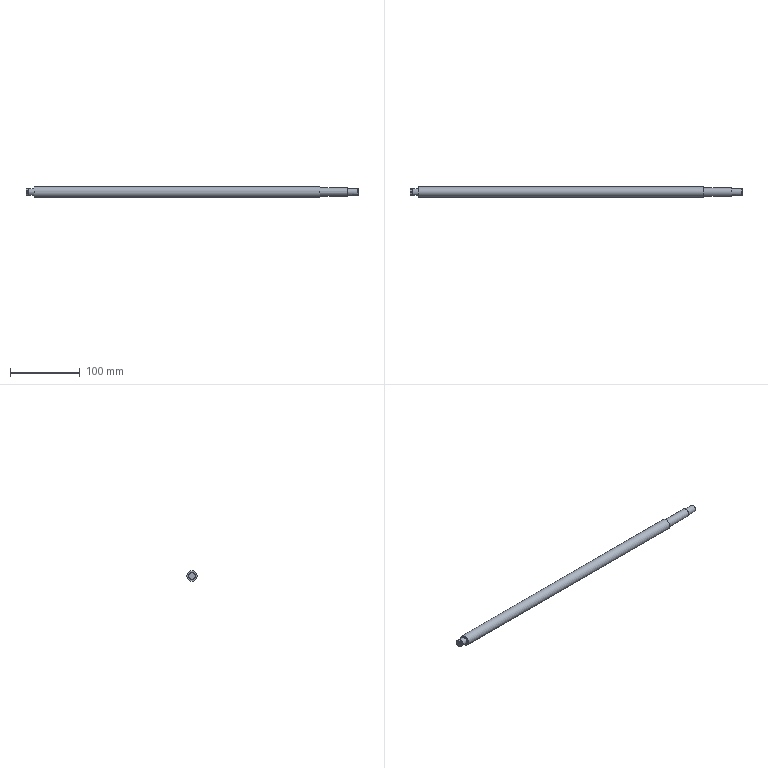Part | STEP file | 1 solid | 17 faces | box 475 x 15 x 15 mm | volume 78728 mm3 | plane 7 | cylinder 6 | spline 2 | cone 2 | commonest cylinder face diameters 10 x3 9.6 x1 12 x1 15 x1
STEP:
#1=CARTESIAN_POINT('',(0.,0.,0.));
#2=DIRECTION('',(0.,0.,1.));
#3=DIRECTION('',(1.,0.,0.));
#4=AXIS2_PLACEMENT_3D('',#1,#2,#3);
#5=CARTESIAN_POINT('',(12.,0.,7.5));
#6=VERTEX_POINT('',#5);
#7=CARTESIAN_POINT('',(12.,0.,0.));
#8=DIRECTION('',(1.,0.,0.));
#9=DIRECTION('',(0.,0.,1.));
#10=AXIS2_PLACEMENT_3D('',#7,#8,#9);
#11=CIRCLE('',#10,7.5);
#12=CARTESIAN_POINT('',(0.,0.,0.));
#13=DIRECTION('',(-1.,0.,0.));
#14=DIRECTION('',(0.,0.,1.));
#15=AXIS2_PLACEMENT_3D('',#12,#13,#14);
#16=CYLINDRICAL_SURFACE('',#15,7.5);
#17=CARTESIAN_POINT('',(6.283,-12.));
#18=DIRECTION('',(-1.,0.));
#19=VECTOR('',#18,1.);
#20=LINE('',#17,#19);
#21=(GEOMETRIC_REPRESENTATION_CONTEXT(2)PARAMETRIC_REPRESENTATION_CONTEXT()REPRESENTATION_CONTEXT('',''));
#22=DEFINITIONAL_REPRESENTATION('',(#20),#21);
#23=PCURVE('',#16,#22);
#24=CARTESIAN_POINT('',(12.,5.,0.));
#25=DIRECTION('',(1.,0.,0.));
#26=DIRECTION('',(0.,0.,-1.));
#27=AXIS2_PLACEMENT_3D('',#24,#25,#26);
#28=PLANE('',#27);
#29=CARTESIAN_POINT('',(0.,-5.));
#30=DIRECTION('',(-1.,0.));
#31=AXIS2_PLACEMENT_2D('',#29,#30);
#32=CIRCLE('',#31,7.5);
#33=(GEOMETRIC_REPRESENTATION_CONTEXT(2)PARAMETRIC_REPRESENTATION_CONTEXT()REPRESENTATION_CONTEXT('',''));
#34=DEFINITIONAL_REPRESENTATION('',(#32),#33);
#35=PCURVE('',#28,#34);
#36=SURFACE_CURVE('',#11,(#23,#35),.PCURVE_S1.);
#37=EDGE_CURVE('',#6,#6,#36,.T.);
#38=ORIENTED_EDGE('',*,*,#37,.T.);
#39=CARTESIAN_POINT('',(420.,0.,7.5));
#40=VERTEX_POINT('',#39);
#41=CARTESIAN_POINT('',(420.,0.,7.5));
#42=CARTESIAN_POINT('',(12.,0.,7.5));
#43=B_SPLINE_CURVE_WITH_KNOTS('',1,(#41,#42),.UNSPECIFIED.,.F.,.F.,(2,2),(-420.,-12.),.PIECEWISE_BEZIER_KNOTS.);
#44=CARTESIAN_POINT('',(0.,0.));
#45=DIRECTION('',(0.,1.));
#46=VECTOR('',#45,1.);
#47=LINE('',#44,#46);
#48=(GEOMETRIC_REPRESENTATION_CONTEXT(2)PARAMETRIC_REPRESENTATION_CONTEXT()REPRESENTATION_CONTEXT('',''));
#49=DEFINITIONAL_REPRESENTATION('',(#47),#48);
#50=PCURVE('',#16,#49);
#51=CARTESIAN_POINT('',(6.283,0.));
#52=DIRECTION('',(0.,1.));
#53=VECTOR('',#52,1.);
#54=LINE('',#51,#53);
#55=(GEOMETRIC_REPRESENTATION_CONTEXT(2)PARAMETRIC_REPRESENTATION_CONTEXT()REPRESENTATION_CONTEXT('',''));
#56=DEFINITIONAL_REPRESENTATION('',(#54),#55);
#57=PCURVE('',#16,#56);
#58=SEAM_CURVE('',#43,(#50,#57),.PCURVE_S1.);
#59=EDGE_CURVE('',#40,#6,#58,.T.);
#60=ORIENTED_EDGE('',*,*,#59,.F.);
#61=CARTESIAN_POINT('',(420.,0.,0.));
#62=DIRECTION('',(-1.,0.,0.));
#63=DIRECTION('',(0.,0.,1.));
#64=AXIS2_PLACEMENT_3D('',#61,#62,#63);
#65=CIRCLE('',#64,7.5);
#66=CARTESIAN_POINT('',(0.,-420.));
#67=DIRECTION('',(1.,0.));
#68=VECTOR('',#67,1.);
#69=LINE('',#66,#68);
#70=(GEOMETRIC_REPRESENTATION_CONTEXT(2)PARAMETRIC_REPRESENTATION_CONTEXT()REPRESENTATION_CONTEXT('',''));
#71=DEFINITIONAL_REPRESENTATION('',(#69),#70);
#72=PCURVE('',#16,#71);
#73=CARTESIAN_POINT('',(420.,6.,0.));
#74=DIRECTION('',(-1.,0.,0.));
#75=DIRECTION('',(0.,0.,1.));
#76=AXIS2_PLACEMENT_3D('',#73,#74,#75);
#77=PLANE('',#76);
#78=CARTESIAN_POINT('',(0.,-6.));
#79=DIRECTION('',(1.,0.));
#80=AXIS2_PLACEMENT_2D('',#78,#79);
#81=CIRCLE('',#80,7.5);
#82=(GEOMETRIC_REPRESENTATION_CONTEXT(2)PARAMETRIC_REPRESENTATION_CONTEXT()REPRESENTATION_CONTEXT('',''));
#83=DEFINITIONAL_REPRESENTATION('',(#81),#82);
#84=PCURVE('',#77,#83);
#85=SURFACE_CURVE('',#65,(#72,#84),.PCURVE_S1.);
#86=EDGE_CURVE('',#40,#40,#85,.T.);
#87=ORIENTED_EDGE('',*,*,#86,.T.);
#88=ORIENTED_EDGE('',*,*,#59,.T.);
#89=EDGE_LOOP('',(#38,#60,#87,#88));
#90=FACE_BOUND('',#89,.T.);
#91=ADVANCED_FACE('',(#90),#16,.T.);
#92=CARTESIAN_POINT('',(12.,0.,-5.3));
#93=VERTEX_POINT('',#92);
#94=CARTESIAN_POINT('',(12.,0.,5.3));
#95=VERTEX_POINT('',#94);
#96=CARTESIAN_POINT('',(12.,0.,-5.3));
#97=CARTESIAN_POINT('',(12.,-10.6,-5.3));
#98=CARTESIAN_POINT('',(12.,-10.6,5.3));
#99=CARTESIAN_POINT('',(12.,0.,5.3));
#100=(BOUNDED_CURVE()B_SPLINE_CURVE(3,(#96,#97,#98,#99),.UNSPECIFIED.,.F.,.F.)B_SPLINE_CURVE_WITH_KNOTS((4,4),(0.,1.),.PIECEWISE_BEZIER_KNOTS.)CURVE()GEOMETRIC_REPRESENTATION_ITEM()RATIONAL_B_SPLINE_CURVE((1.,0.3333,0.3333,1.))REPRESENTATION_ITEM(''));
#101=CARTESIAN_POINT('',(5.3,-5.));
#102=CARTESIAN_POINT('',(5.3,-15.6));
#103=CARTESIAN_POINT('',(-5.3,-15.6));
#104=CARTESIAN_POINT('',(-5.3,-5.));
#105=(BOUNDED_CURVE()B_SPLINE_CURVE(3,(#101,#102,#103,#104),.UNSPECIFIED.,.F.,.F.)B_SPLINE_CURVE_WITH_KNOTS((4,4),(0.,1.),.PIECEWISE_BEZIER_KNOTS.)CURVE()GEOMETRIC_REPRESENTATION_ITEM()RATIONAL_B_SPLINE_CURVE((1.,0.3333,0.3333,1.))REPRESENTATION_ITEM(''));
#106=(GEOMETRIC_REPRESENTATION_CONTEXT(2)PARAMETRIC_REPRESENTATION_CONTEXT()REPRESENTATION_CONTEXT('',''));
#107=DEFINITIONAL_REPRESENTATION('',(#105),#106);
#108=PCURVE('',#28,#107);
#109=CARTESIAN_POINT('',(11.7,0.,-5.));
#110=CARTESIAN_POINT('',(11.7,10.,-5.));
#111=CARTESIAN_POINT('',(11.7,10.,5.));
#112=CARTESIAN_POINT('',(11.7,0.,5.));
#113=CARTESIAN_POINT('',(11.7,-10.,5.));
#114=CARTESIAN_POINT('',(11.7,-10.,-5.));
#115=CARTESIAN_POINT('',(11.7,0.,-5.));
#116=CARTESIAN_POINT('',(11.876,0.,-5.));
#117=CARTESIAN_POINT('',(11.876,10.,-5.));
#118=CARTESIAN_POINT('',(11.876,10.,5.));
#119=CARTESIAN_POINT('',(11.876,0.,5.));
#120=CARTESIAN_POINT('',(11.876,-10.,5.));
#121=CARTESIAN_POINT('',(11.876,-10.,-5.));
#122=CARTESIAN_POINT('',(11.876,0.,-5.));
#123=CARTESIAN_POINT('',(12.,0.,-5.124));
#124=CARTESIAN_POINT('',(12.,10.249,-5.124));
#125=CARTESIAN_POINT('',(12.,10.249,5.124));
#126=CARTESIAN_POINT('',(12.,0.,5.124));
#127=CARTESIAN_POINT('',(12.,-10.249,5.124));
#128=CARTESIAN_POINT('',(12.,-10.249,-5.124));
#129=CARTESIAN_POINT('',(12.,0.,-5.124));
#130=CARTESIAN_POINT('',(12.,0.,-5.3));
#131=CARTESIAN_POINT('',(12.,10.6,-5.3));
#132=CARTESIAN_POINT('',(12.,10.6,5.3));
#133=CARTESIAN_POINT('',(12.,0.,5.3));
#134=CARTESIAN_POINT('',(12.,-10.6,5.3));
#135=CARTESIAN_POINT('',(12.,-10.6,-5.3));
#136=CARTESIAN_POINT('',(12.,0.,-5.3));
#137=(BOUNDED_SURFACE()B_SPLINE_SURFACE(3,3,((#109,#110,#111,#112,#113,#114,#115),(#116,#117,#118,#119,#120,#121,#122),(#123,#124,#125,#126,#127,#128,#129),(#130,#131,#132,#133,#134,#135,#136)),.UNSPECIFIED.,.F.,.T.,.F.)B_SPLINE_SURFACE_WITH_KNOTS((4,4),(1,3,3,3,1),(0.,1.),(-0.5,0.,0.5,1.,1.5),.UNSPECIFIED.)GEOMETRIC_REPRESENTATION_ITEM()RATIONAL_B_SPLINE_SURFACE(((1.,0.3333,0.3333,1.,0.3333,0.3333,1.),(0.8047,0.2682,0.2682,0.8047,0.2682,0.2682,0.8047),(0.8047,0.2682,0.2682,0.8047,0.2682,0.2682,0.8047),(1.,0.3333,0.3333,1.,0.3333,0.3333,1.)))REPRESENTATION_ITEM('')SURFACE());
#138=CARTESIAN_POINT('',(1.,1.));
#139=CARTESIAN_POINT('',(1.,0.5));
#140=B_SPLINE_CURVE_WITH_KNOTS('',1,(#138,#139),.UNSPECIFIED.,.F.,.F.,(2,2),(0.,1.),.PIECEWISE_BEZIER_KNOTS.);
#141=(GEOMETRIC_REPRESENTATION_CONTEXT(2)PARAMETRIC_REPRESENTATION_CONTEXT()REPRESENTATION_CONTEXT('',''));
#142=DEFINITIONAL_REPRESENTATION('',(#140),#141);
#143=PCURVE('',#137,#142);
#144=SURFACE_CURVE('',#100,(#108,#143),.PCURVE_S1.);
#145=EDGE_CURVE('',#93,#95,#144,.T.);
#146=ORIENTED_EDGE('',*,*,#145,.F.);
#147=CARTESIAN_POINT('',(12.,0.,5.3));
#148=CARTESIAN_POINT('',(12.,10.6,5.3));
#149=CARTESIAN_POINT('',(12.,10.6,-5.3));
#150=CARTESIAN_POINT('',(12.,0.,-5.3));
#151=(BOUNDED_CURVE()B_SPLINE_CURVE(3,(#147,#148,#149,#150),.UNSPECIFIED.,.F.,.F.)B_SPLINE_CURVE_WITH_KNOTS((4,4),(0.,1.),.PIECEWISE_BEZIER_KNOTS.)CURVE()GEOMETRIC_REPRESENTATION_ITEM()RATIONAL_B_SPLINE_CURVE((1.,0.3333,0.3333,1.))REPRESENTATION_ITEM(''));
#152=CARTESIAN_POINT('',(-5.3,-5.));
#153=CARTESIAN_POINT('',(-5.3,5.6));
#154=CARTESIAN_POINT('',(5.3,5.6));
#155=CARTESIAN_POINT('',(5.3,-5.));
#156=(BOUNDED_CURVE()B_SPLINE_CURVE(3,(#152,#153,#154,#155),.UNSPECIFIED.,.F.,.F.)B_SPLINE_CURVE_WITH_KNOTS((4,4),(0.,1.),.PIECEWISE_BEZIER_KNOTS.)CURVE()GEOMETRIC_REPRESENTATION_ITEM()RATIONAL_B_SPLINE_CURVE((1.,0.3333,0.3333,1.))REPRESENTATION_ITEM(''));
#157=(GEOMETRIC_REPRESENTATION_CONTEXT(2)PARAMETRIC_REPRESENTATION_CONTEXT()REPRESENTATION_CONTEXT('',''));
#158=DEFINITIONAL_REPRESENTATION('',(#156),#157);
#159=PCURVE('',#28,#158);
#160=CARTESIAN_POINT('',(1.,0.5));
#161=CARTESIAN_POINT('',(1.,0.));
#162=B_SPLINE_CURVE_WITH_KNOTS('',1,(#160,#161),.UNSPECIFIED.,.F.,.F.,(2,2),(0.,1.),.PIECEWISE_BEZIER_KNOTS.);
#163=(GEOMETRIC_REPRESENTATION_CONTEXT(2)PARAMETRIC_REPRESENTATION_CONTEXT()REPRESENTATION_CONTEXT('',''));
#164=DEFINITIONAL_REPRESENTATION('',(#162),#163);
#165=PCURVE('',#137,#164);
#166=SURFACE_CURVE('',#151,(#159,#165),.PCURVE_S1.);
#167=EDGE_CURVE('',#95,#93,#166,.T.);
#168=ORIENTED_EDGE('',*,*,#167,.F.);
#169=EDGE_LOOP('',(#146,#168));
#170=FACE_BOUND('',#169,.T.);
#171=ORIENTED_EDGE('',*,*,#37,.F.);
#172=EDGE_LOOP('',(#171));
#173=FACE_BOUND('',#172,.T.);
#174=ADVANCED_FACE('',(#170,#173),#28,.F.);
#175=CARTESIAN_POINT('',(420.,0.,6.3));
#176=VERTEX_POINT('',#175);
#177=CARTESIAN_POINT('',(420.,0.,-6.3));
#178=VERTEX_POINT('',#177);
#179=CARTESIAN_POINT('',(420.,0.,6.3));
#180=CARTESIAN_POINT('',(420.,-12.6,6.3));
#181=CARTESIAN_POINT('',(420.,-12.6,-6.3));
#182=CARTESIAN_POINT('',(420.,0.,-6.3));
#183=(BOUNDED_CURVE()B_SPLINE_CURVE(3,(#179,#180,#181,#182),.UNSPECIFIED.,.F.,.F.)B_SPLINE_CURVE_WITH_KNOTS((4,4),(0.,1.),.PIECEWISE_BEZIER_KNOTS.)CURVE()GEOMETRIC_REPRESENTATION_ITEM()RATIONAL_B_SPLINE_CURVE((1.,0.3333,0.3333,1.))REPRESENTATION_ITEM(''));
#184=CARTESIAN_POINT('',(6.3,-6.));
#185=CARTESIAN_POINT('',(6.3,-18.6));
#186=CARTESIAN_POINT('',(-6.3,-18.6));
#187=CARTESIAN_POINT('',(-6.3,-6.));
#188=(BOUNDED_CURVE()B_SPLINE_CURVE(3,(#184,#185,#186,#187),.UNSPECIFIED.,.F.,.F.)B_SPLINE_CURVE_WITH_KNOTS((4,4),(0.,1.),.PIECEWISE_BEZIER_KNOTS.)CURVE()GEOMETRIC_REPRESENTATION_ITEM()RATIONAL_B_SPLINE_CURVE((1.,0.3333,0.3333,1.))REPRESENTATION_ITEM(''));
#189=(GEOMETRIC_REPRESENTATION_CONTEXT(2)PARAMETRIC_REPRESENTATION_CONTEXT()REPRESENTATION_CONTEXT('',''));
#190=DEFINITIONAL_REPRESENTATION('',(#188),#189);
#191=PCURVE('',#77,#190);
#192=CARTESIAN_POINT('',(420.3,0.,6.));
#193=CARTESIAN_POINT('',(420.3,12.,6.));
#194=CARTESIAN_POINT('',(420.3,12.,-6.));
#195=CARTESIAN_POINT('',(420.3,0.,-6.));
#196=CARTESIAN_POINT('',(420.3,-12.,-6.));
#197=CARTESIAN_POINT('',(420.3,-12.,6.));
#198=CARTESIAN_POINT('',(420.3,0.,6.));
#199=CARTESIAN_POINT('',(420.124,0.,6.));
#200=CARTESIAN_POINT('',(420.124,12.,6.));
#201=CARTESIAN_POINT('',(420.124,12.,-6.));
#202=CARTESIAN_POINT('',(420.124,0.,-6.));
#203=CARTESIAN_POINT('',(420.124,-12.,-6.));
#204=CARTESIAN_POINT('',(420.124,-12.,6.));
#205=CARTESIAN_POINT('',(420.124,0.,6.));
#206=CARTESIAN_POINT('',(420.,0.,6.124));
#207=CARTESIAN_POINT('',(420.,12.249,6.124));
#208=CARTESIAN_POINT('',(420.,12.249,-6.124));
#209=CARTESIAN_POINT('',(420.,0.,-6.124));
#210=CARTESIAN_POINT('',(420.,-12.249,-6.124));
#211=CARTESIAN_POINT('',(420.,-12.249,6.124));
#212=CARTESIAN_POINT('',(420.,0.,6.124));
#213=CARTESIAN_POINT('',(420.,0.,6.3));
#214=CARTESIAN_POINT('',(420.,12.6,6.3));
#215=CARTESIAN_POINT('',(420.,12.6,-6.3));
#216=CARTESIAN_POINT('',(420.,0.,-6.3));
#217=CARTESIAN_POINT('',(420.,-12.6,-6.3));
#218=CARTESIAN_POINT('',(420.,-12.6,6.3));
#219=CARTESIAN_POINT('',(420.,0.,6.3));
#220=(BOUNDED_SURFACE()B_SPLINE_SURFACE(3,3,((#192,#193,#194,#195,#196,#197,#198),(#199,#200,#201,#202,#203,#204,#205),(#206,#207,#208,#209,#210,#211,#212),(#213,#214,#215,#216,#217,#218,#219)),.UNSPECIFIED.,.F.,.T.,.F.)B_SPLINE_SURFACE_WITH_KNOTS((4,4),(1,3,3,3,1),(0.,1.),(-0.5,0.,0.5,1.,1.5),.UNSPECIFIED.)GEOMETRIC_REPRESENTATION_ITEM()RATIONAL_B_SPLINE_SURFACE(((1.,0.3333,0.3333,1.,0.3333,0.3333,1.),(0.8047,0.2682,0.2682,0.8047,0.2682,0.2682,0.8047),(0.8047,0.2682,0.2682,0.8047,0.2682,0.2682,0.8047),(1.,0.3333,0.3333,1.,0.3333,0.3333,1.)))REPRESENTATION_ITEM('')SURFACE());
#221=CARTESIAN_POINT('',(1.,1.));
#222=CARTESIAN_POINT('',(1.,0.5));
#223=B_SPLINE_CURVE_WITH_KNOTS('',1,(#221,#222),.UNSPECIFIED.,.F.,.F.,(2,2),(0.,1.),.PIECEWISE_BEZIER_KNOTS.);
#224=(GEOMETRIC_REPRESENTATION_CONTEXT(2)PARAMETRIC_REPRESENTATION_CONTEXT()REPRESENTATION_CONTEXT('',''));
#225=DEFINITIONAL_REPRESENTATION('',(#223),#224);
#226=PCURVE('',#220,#225);
#227=SURFACE_CURVE('',#183,(#191,#226),.PCURVE_S1.);
#228=EDGE_CURVE('',#176,#178,#227,.T.);
#229=ORIENTED_EDGE('',*,*,#228,.F.);
#230=CARTESIAN_POINT('',(420.,0.,-6.3));
#231=CARTESIAN_POINT('',(420.,12.6,-6.3));
#232=CARTESIAN_POINT('',(420.,12.6,6.3));
#233=CARTESIAN_POINT('',(420.,0.,6.3));
#234=(BOUNDED_CURVE()B_SPLINE_CURVE(3,(#230,#231,#232,#233),.UNSPECIFIED.,.F.,.F.)B_SPLINE_CURVE_WITH_KNOTS((4,4),(0.,1.),.PIECEWISE_BEZIER_KNOTS.)CURVE()GEOMETRIC_REPRESENTATION_ITEM()RATIONAL_B_SPLINE_CURVE((1.,0.3333,0.3333,1.))REPRESENTATION_ITEM(''));
#235=CARTESIAN_POINT('',(-6.3,-6.));
#236=CARTESIAN_POINT('',(-6.3,6.6));
#237=CARTESIAN_POINT('',(6.3,6.6));
#238=CARTESIAN_POINT('',(6.3,-6.));
#239=(BOUNDED_CURVE()B_SPLINE_CURVE(3,(#235,#236,#237,#238),.UNSPECIFIED.,.F.,.F.)B_SPLINE_CURVE_WITH_KNOTS((4,4),(0.,1.),.PIECEWISE_BEZIER_KNOTS.)CURVE()GEOMETRIC_REPRESENTATION_ITEM()RATIONAL_B_SPLINE_CURVE((1.,0.3333,0.3333,1.))REPRESENTATION_ITEM(''));
#240=(GEOMETRIC_REPRESENTATION_CONTEXT(2)PARAMETRIC_REPRESENTATION_CONTEXT()REPRESENTATION_CONTEXT('',''));
#241=DEFINITIONAL_REPRESENTATION('',(#239),#240);
#242=PCURVE('',#77,#241);
#243=CARTESIAN_POINT('',(1.,0.5));
#244=CARTESIAN_POINT('',(1.,0.));
#245=B_SPLINE_CURVE_WITH_KNOTS('',1,(#243,#244),.UNSPECIFIED.,.F.,.F.,(2,2),(0.,1.),.PIECEWISE_BEZIER_KNOTS.);
#246=(GEOMETRIC_REPRESENTATION_CONTEXT(2)PARAMETRIC_REPRESENTATION_CONTEXT()REPRESENTATION_CONTEXT('',''));
#247=DEFINITIONAL_REPRESENTATION('',(#245),#246);
#248=PCURVE('',#220,#247);
#249=SURFACE_CURVE('',#234,(#242,#248),.PCURVE_S1.);
#250=EDGE_CURVE('',#178,#176,#249,.T.);
#251=ORIENTED_EDGE('',*,*,#250,.F.);
#252=EDGE_LOOP('',(#229,#251));
#253=FACE_BOUND('',#252,.T.);
#254=ORIENTED_EDGE('',*,*,#86,.F.);
#255=EDGE_LOOP('',(#254));
#256=FACE_BOUND('',#255,.T.);
#257=ADVANCED_FACE('',(#253,#256),#77,.F.);
#258=ORIENTED_EDGE('',*,*,#145,.F.);
#259=CARTESIAN_POINT('',(11.7,0.,-5.));
#260=VERTEX_POINT('',#259);
#261=CARTESIAN_POINT('',(11.7,0.,-5.));
#262=CARTESIAN_POINT('',(11.876,0.,-5.));
#263=CARTESIAN_POINT('',(12.,0.,-5.124));
#264=CARTESIAN_POINT('',(12.,0.,-5.3));
#265=(BOUNDED_CURVE()B_SPLINE_CURVE(3,(#261,#262,#263,#264),.UNSPECIFIED.,.F.,.F.)B_SPLINE_CURVE_WITH_KNOTS((4,4),(0.,1.),.PIECEWISE_BEZIER_KNOTS.)CURVE()GEOMETRIC_REPRESENTATION_ITEM()RATIONAL_B_SPLINE_CURVE((1.,0.8047,0.8047,1.))REPRESENTATION_ITEM(''));
#266=CARTESIAN_POINT('',(0.,1.));
#267=DIRECTION('',(1.,0.));
#268=VECTOR('',#267,1.);
#269=LINE('',#266,#268);
#270=(GEOMETRIC_REPRESENTATION_CONTEXT(2)PARAMETRIC_REPRESENTATION_CONTEXT()REPRESENTATION_CONTEXT('',''));
#271=DEFINITIONAL_REPRESENTATION('',(#269),#270);
#272=PCURVE('',#137,#271);
#273=CARTESIAN_POINT('',(0.,0.));
#274=DIRECTION('',(1.,0.));
#275=VECTOR('',#274,1.);
#276=LINE('',#273,#275);
#277=(GEOMETRIC_REPRESENTATION_CONTEXT(2)PARAMETRIC_REPRESENTATION_CONTEXT()REPRESENTATION_CONTEXT('',''));
#278=DEFINITIONAL_REPRESENTATION('',(#276),#277);
#279=PCURVE('',#137,#278);
#280=SEAM_CURVE('',#265,(#272,#279),.PCURVE_S1.);
#281=EDGE_CURVE('',#260,#93,#280,.T.);
#282=ORIENTED_EDGE('',*,*,#281,.F.);
#283=CARTESIAN_POINT('',(11.7,0.,5.));
#284=VERTEX_POINT('',#283);
#285=CARTESIAN_POINT('',(11.7,0.,0.));
#286=DIRECTION('',(-1.,0.,0.));
#287=DIRECTION('',(0.,0.,-1.));
#288=AXIS2_PLACEMENT_3D('',#285,#286,#287);
#289=CIRCLE('',#288,5.);
#290=CARTESIAN_POINT('',(0.,1.));
#291=CARTESIAN_POINT('',(0.,0.9765));
#292=CARTESIAN_POINT('',(0.,0.9351));
#293=CARTESIAN_POINT('',(0.,0.8854));
#294=CARTESIAN_POINT('',(0.,0.8425));
#295=CARTESIAN_POINT('',(0.,0.804));
#296=CARTESIAN_POINT('',(0.,0.7678));
#297=CARTESIAN_POINT('',(0.,0.7322));
#298=CARTESIAN_POINT('',(0.,0.696));
#299=CARTESIAN_POINT('',(0.,0.6575));
#300=CARTESIAN_POINT('',(0.,0.6144));
#301=CARTESIAN_POINT('',(0.,0.5657));
#302=CARTESIAN_POINT('',(0.,0.5));
#303=CARTESIAN_POINT('',(0.,0.4343));
#304=CARTESIAN_POINT('',(0.,0.3856));
#305=CARTESIAN_POINT('',(0.,0.3425));
#306=CARTESIAN_POINT('',(0.,0.304));
#307=CARTESIAN_POINT('',(0.,0.2678));
#308=CARTESIAN_POINT('',(0.,0.2322));
#309=CARTESIAN_POINT('',(0.,0.196));
#310=CARTESIAN_POINT('',(0.,0.1575));
#311=CARTESIAN_POINT('',(0.,0.1146));
#312=CARTESIAN_POINT('',(0.,0.06491));
#313=CARTESIAN_POINT('',(0.,0.02352));
#314=CARTESIAN_POINT('',(0.,0.));
#315=B_SPLINE_CURVE_WITH_KNOTS('',3,(#290,#291,#292,#293,#294,#295,#296,#297,#298,#299,#300,#301,#302,#303,#304,#305,#306,#307,#308,#309,#310,#311,#312,#313,#314),.UNSPECIFIED.,.F.,.F.,(4,1,1,1,1,1,1,1,1,1,1,1,1,1,1,1,1,1,1,1,1,1,4),(0.,0.2856,0.5712,0.8568,1.142,1.428,1.714,1.999,2.285,2.57,2.856,3.142,3.427,3.713,3.998,4.284,4.57,4.855,5.141,5.426,5.712,5.998,6.283),.QUASI_UNIFORM_KNOTS.);
#316=(GEOMETRIC_REPRESENTATION_CONTEXT(2)PARAMETRIC_REPRESENTATION_CONTEXT()REPRESENTATION_CONTEXT('',''));
#317=DEFINITIONAL_REPRESENTATION('',(#315),#316);
#318=PCURVE('',#137,#317);
#319=CARTESIAN_POINT('',(0.,0.,0.));
#320=DIRECTION('',(-1.,0.,0.));
#321=DIRECTION('',(0.,0.,1.));
#322=AXIS2_PLACEMENT_3D('',#319,#320,#321);
#323=CYLINDRICAL_SURFACE('',#322,5.);
#324=CARTESIAN_POINT('',(3.142,-11.7));
#325=DIRECTION('',(1.,0.));
#326=VECTOR('',#325,1.);
#327=LINE('',#324,#326);
#328=(GEOMETRIC_REPRESENTATION_CONTEXT(2)PARAMETRIC_REPRESENTATION_CONTEXT()REPRESENTATION_CONTEXT('',''));
#329=DEFINITIONAL_REPRESENTATION('',(#327),#328);
#330=PCURVE('',#323,#329);
#331=SURFACE_CURVE('',#289,(#318,#330),.PCURVE_S1.);
#332=EDGE_CURVE('',#260,#284,#331,.T.);
#333=ORIENTED_EDGE('',*,*,#332,.T.);
#334=CARTESIAN_POINT('',(11.7,0.,0.));
#335=DIRECTION('',(-1.,0.,0.));
#336=DIRECTION('',(0.,0.,-1.));
#337=AXIS2_PLACEMENT_3D('',#334,#335,#336);
#338=CIRCLE('',#337,5.);
#339=CARTESIAN_POINT('',(0.,1.));
#340=CARTESIAN_POINT('',(0.,0.9765));
#341=CARTESIAN_POINT('',(0.,0.9351));
#342=CARTESIAN_POINT('',(0.,0.8854));
#343=CARTESIAN_POINT('',(0.,0.8425));
#344=CARTESIAN_POINT('',(0.,0.804));
#345=CARTESIAN_POINT('',(0.,0.7678));
#346=CARTESIAN_POINT('',(0.,0.7322));
#347=CARTESIAN_POINT('',(0.,0.696));
#348=CARTESIAN_POINT('',(0.,0.6575));
#349=CARTESIAN_POINT('',(0.,0.6144));
#350=CARTESIAN_POINT('',(0.,0.5657));
#351=CARTESIAN_POINT('',(0.,0.5));
#352=CARTESIAN_POINT('',(0.,0.4343));
#353=CARTESIAN_POINT('',(0.,0.3856));
#354=CARTESIAN_POINT('',(0.,0.3425));
#355=CARTESIAN_POINT('',(0.,0.304));
#356=CARTESIAN_POINT('',(0.,0.2678));
#357=CARTESIAN_POINT('',(0.,0.2322));
#358=CARTESIAN_POINT('',(0.,0.196));
#359=CARTESIAN_POINT('',(0.,0.1575));
#360=CARTESIAN_POINT('',(0.,0.1146));
#361=CARTESIAN_POINT('',(0.,0.06491));
#362=CARTESIAN_POINT('',(0.,0.02352));
#363=CARTESIAN_POINT('',(0.,0.));
#364=B_SPLINE_CURVE_WITH_KNOTS('',3,(#339,#340,#341,#342,#343,#344,#345,#346,#347,#348,#349,#350,#351,#352,#353,#354,#355,#356,#357,#358,#359,#360,#361,#362,#363),.UNSPECIFIED.,.F.,.F.,(4,1,1,1,1,1,1,1,1,1,1,1,1,1,1,1,1,1,1,1,1,1,4),(0.,0.2856,0.5712,0.8568,1.142,1.428,1.714,1.999,2.285,2.57,2.856,3.142,3.427,3.713,3.998,4.284,4.57,4.855,5.141,5.426,5.712,5.998,6.283),.QUASI_UNIFORM_KNOTS.);
#365=(GEOMETRIC_REPRESENTATION_CONTEXT(2)PARAMETRIC_REPRESENTATION_CONTEXT()REPRESENTATION_CONTEXT('',''));
#366=DEFINITIONAL_REPRESENTATION('',(#364),#365);
#367=PCURVE('',#137,#366);
#368=CARTESIAN_POINT('',(-3.142,-11.7));
#369=DIRECTION('',(1.,0.));
#370=VECTOR('',#369,1.);
#371=LINE('',#368,#370);
#372=(GEOMETRIC_REPRESENTATION_CONTEXT(2)PARAMETRIC_REPRESENTATION_CONTEXT()REPRESENTATION_CONTEXT('',''));
#373=DEFINITIONAL_REPRESENTATION('',(#371),#372);
#374=PCURVE('',#323,#373);
#375=SURFACE_CURVE('',#338,(#367,#374),.PCURVE_S1.);
#376=EDGE_CURVE('',#284,#260,#375,.T.);
#377=ORIENTED_EDGE('',*,*,#376,.T.);
#378=ORIENTED_EDGE('',*,*,#281,.T.);
#379=ORIENTED_EDGE('',*,*,#167,.F.);
#380=EDGE_LOOP('',(#258,#282,#333,#377,#378,#379));
#381=FACE_BOUND('',#380,.F.);
#382=ADVANCED_FACE('',(#381),#137,.F.);
#383=ORIENTED_EDGE('',*,*,#228,.F.);
#384=CARTESIAN_POINT('',(420.3,0.,6.));
#385=VERTEX_POINT('',#384);
#386=CARTESIAN_POINT('',(420.3,0.,6.));
#387=CARTESIAN_POINT('',(420.124,0.,6.));
#388=CARTESIAN_POINT('',(420.,0.,6.124));
#389=CARTESIAN_POINT('',(420.,0.,6.3));
#390=(BOUNDED_CURVE()B_SPLINE_CURVE(3,(#386,#387,#388,#389),.UNSPECIFIED.,.F.,.F.)B_SPLINE_CURVE_WITH_KNOTS((4,4),(0.,1.),.PIECEWISE_BEZIER_KNOTS.)CURVE()GEOMETRIC_REPRESENTATION_ITEM()RATIONAL_B_SPLINE_CURVE((1.,0.8047,0.8047,1.))REPRESENTATION_ITEM(''));
#391=CARTESIAN_POINT('',(0.,1.));
#392=DIRECTION('',(1.,0.));
#393=VECTOR('',#392,1.);
#394=LINE('',#391,#393);
#395=(GEOMETRIC_REPRESENTATION_CONTEXT(2)PARAMETRIC_REPRESENTATION_CONTEXT()REPRESENTATION_CONTEXT('',''));
#396=DEFINITIONAL_REPRESENTATION('',(#394),#395);
#397=PCURVE('',#220,#396);
#398=CARTESIAN_POINT('',(0.,0.));
#399=DIRECTION('',(1.,0.));
#400=VECTOR('',#399,1.);
#401=LINE('',#398,#400);
#402=(GEOMETRIC_REPRESENTATION_CONTEXT(2)PARAMETRIC_REPRESENTATION_CONTEXT()REPRESENTATION_CONTEXT('',''));
#403=DEFINITIONAL_REPRESENTATION('',(#401),#402);
#404=PCURVE('',#220,#403);
#405=SEAM_CURVE('',#390,(#397,#404),.PCURVE_S1.);
#406=EDGE_CURVE('',#385,#176,#405,.T.);
#407=ORIENTED_EDGE('',*,*,#406,.F.);
#408=CARTESIAN_POINT('',(420.3,0.,0.));
#409=DIRECTION('',(1.,0.,0.));
#410=DIRECTION('',(0.,0.,1.));
#411=AXIS2_PLACEMENT_3D('',#408,#409,#410);
#412=CIRCLE('',#411,6.);
#413=CARTESIAN_POINT('',(0.,1.));
#414=CARTESIAN_POINT('',(0.,0.9765));
#415=CARTESIAN_POINT('',(0.,0.9351));
#416=CARTESIAN_POINT('',(0.,0.8854));
#417=CARTESIAN_POINT('',(0.,0.8425));
#418=CARTESIAN_POINT('',(0.,0.804));
#419=CARTESIAN_POINT('',(0.,0.7678));
#420=CARTESIAN_POINT('',(0.,0.7322));
#421=CARTESIAN_POINT('',(0.,0.696));
#422=CARTESIAN_POINT('',(0.,0.6575));
#423=CARTESIAN_POINT('',(0.,0.6144));
#424=CARTESIAN_POINT('',(0.,0.5657));
#425=CARTESIAN_POINT('',(0.,0.5));
#426=CARTESIAN_POINT('',(0.,0.4343));
#427=CARTESIAN_POINT('',(0.,0.3856));
#428=CARTESIAN_POINT('',(0.,0.3425));
#429=CARTESIAN_POINT('',(0.,0.304));
#430=CARTESIAN_POINT('',(0.,0.2678));
#431=CARTESIAN_POINT('',(0.,0.2322));
#432=CARTESIAN_POINT('',(0.,0.196));
#433=CARTESIAN_POINT('',(0.,0.1575));
#434=CARTESIAN_POINT('',(0.,0.1146));
#435=CARTESIAN_POINT('',(0.,0.06491));
#436=CARTESIAN_POINT('',(0.,0.02352));
#437=CARTESIAN_POINT('',(0.,0.));
#438=B_SPLINE_CURVE_WITH_KNOTS('',3,(#413,#414,#415,#416,#417,#418,#419,#420,#421,#422,#423,#424,#425,#426,#427,#428,#429,#430,#431,#432,#433,#434,#435,#436,#437),.UNSPECIFIED.,.F.,.F.,(4,1,1,1,1,1,1,1,1,1,1,1,1,1,1,1,1,1,1,1,1,1,4),(0.,0.2856,0.5712,0.8568,1.142,1.428,1.714,1.999,2.285,2.57,2.856,3.142,3.427,3.713,3.998,4.284,4.57,4.855,5.141,5.426,5.712,5.998,6.283),.QUASI_UNIFORM_KNOTS.);
#439=(GEOMETRIC_REPRESENTATION_CONTEXT(2)PARAMETRIC_REPRESENTATION_CONTEXT()REPRESENTATION_CONTEXT('',''));
#440=DEFINITIONAL_REPRESENTATION('',(#438),#439);
#441=PCURVE('',#220,#440);
#442=CARTESIAN_POINT('',(0.,0.,0.));
#443=DIRECTION('',(-1.,0.,0.));
#444=DIRECTION('',(0.,0.,1.));
#445=AXIS2_PLACEMENT_3D('',#442,#443,#444);
#446=CYLINDRICAL_SURFACE('',#445,6.);
#447=CARTESIAN_POINT('',(6.283,-420.3));
#448=DIRECTION('',(-1.,0.));
#449=VECTOR('',#448,1.);
#450=LINE('',#447,#449);
#451=(GEOMETRIC_REPRESENTATION_CONTEXT(2)PARAMETRIC_REPRESENTATION_CONTEXT()REPRESENTATION_CONTEXT('',''));
#452=DEFINITIONAL_REPRESENTATION('',(#450),#451);
#453=PCURVE('',#446,#452);
#454=SURFACE_CURVE('',#412,(#441,#453),.PCURVE_S1.);
#455=EDGE_CURVE('',#385,#385,#454,.T.);
#456=ORIENTED_EDGE('',*,*,#455,.T.);
#457=ORIENTED_EDGE('',*,*,#406,.T.);
#458=ORIENTED_EDGE('',*,*,#250,.F.);
#459=EDGE_LOOP('',(#383,#407,#456,#457,#458));
#460=FACE_BOUND('',#459,.F.);
#461=ADVANCED_FACE('',(#460),#220,.F.);
#462=CARTESIAN_POINT('',(4.,0.,5.));
#463=VERTEX_POINT('',#462);
#464=CARTESIAN_POINT('',(4.,0.,0.));
#465=DIRECTION('',(1.,0.,0.));
#466=DIRECTION('',(0.,0.,1.));
#467=AXIS2_PLACEMENT_3D('',#464,#465,#466);
#468=CIRCLE('',#467,5.);
#469=CARTESIAN_POINT('',(6.283,-4.));
#470=DIRECTION('',(-1.,0.));
#471=VECTOR('',#470,1.);
#472=LINE('',#469,#471);
#473=(GEOMETRIC_REPRESENTATION_CONTEXT(2)PARAMETRIC_REPRESENTATION_CONTEXT()REPRESENTATION_CONTEXT('',''));
#474=DEFINITIONAL_REPRESENTATION('',(#472),#473);
#475=PCURVE('',#323,#474);
#476=CARTESIAN_POINT('',(4.,5.,0.));
#477=DIRECTION('',(-1.,0.,0.));
#478=DIRECTION('',(0.,0.,1.));
#479=AXIS2_PLACEMENT_3D('',#476,#477,#478);
#480=PLANE('',#479);
#481=CARTESIAN_POINT('',(5.,-5.));
#482=CARTESIAN_POINT('',(5.,-13.66));
#483=CARTESIAN_POINT('',(-2.5,-9.33));
#484=CARTESIAN_POINT('',(-10.,-5.));
#485=CARTESIAN_POINT('',(-2.5,-0.6699));
#486=CARTESIAN_POINT('',(5.,3.66));
#487=CARTESIAN_POINT('',(5.,-5.));
#488=(BOUNDED_CURVE()B_SPLINE_CURVE(2,(#481,#482,#483,#484,#485,#486,#487),.UNSPECIFIED.,.T.,.F.)B_SPLINE_CURVE_WITH_KNOTS((1,2,2,2,2,1),(-2.094,0.,2.094,4.189,6.283,8.378),.UNSPECIFIED.)CURVE()GEOMETRIC_REPRESENTATION_ITEM()RATIONAL_B_SPLINE_CURVE((1.,0.5,1.,0.5,1.,0.5,1.))REPRESENTATION_ITEM(''));
#489=(GEOMETRIC_REPRESENTATION_CONTEXT(2)PARAMETRIC_REPRESENTATION_CONTEXT()REPRESENTATION_CONTEXT('',''));
#490=DEFINITIONAL_REPRESENTATION('',(#488),#489);
#491=PCURVE('',#480,#490);
#492=SURFACE_CURVE('',#468,(#475,#491),.PCURVE_S1.);
#493=EDGE_CURVE('',#463,#463,#492,.T.);
#494=ORIENTED_EDGE('',*,*,#493,.T.);
#495=CARTESIAN_POINT('',(11.7,0.,5.));
#496=CARTESIAN_POINT('',(4.,0.,5.));
#497=B_SPLINE_CURVE_WITH_KNOTS('',1,(#495,#496),.UNSPECIFIED.,.F.,.F.,(2,2),(-11.7,-4.),.PIECEWISE_BEZIER_KNOTS.);
#498=CARTESIAN_POINT('',(0.,0.));
#499=DIRECTION('',(0.,1.));
#500=VECTOR('',#499,1.);
#501=LINE('',#498,#500);
#502=(GEOMETRIC_REPRESENTATION_CONTEXT(2)PARAMETRIC_REPRESENTATION_CONTEXT()REPRESENTATION_CONTEXT('',''));
#503=DEFINITIONAL_REPRESENTATION('',(#501),#502);
#504=PCURVE('',#323,#503);
#505=CARTESIAN_POINT('',(6.283,0.));
#506=DIRECTION('',(0.,1.));
#507=VECTOR('',#506,1.);
#508=LINE('',#505,#507);
#509=(GEOMETRIC_REPRESENTATION_CONTEXT(2)PARAMETRIC_REPRESENTATION_CONTEXT()REPRESENTATION_CONTEXT('',''));
#510=DEFINITIONAL_REPRESENTATION('',(#508),#509);
#511=PCURVE('',#323,#510);
#512=SEAM_CURVE('',#497,(#504,#511),.PCURVE_S1.);
#513=EDGE_CURVE('',#284,#463,#512,.T.);
#514=ORIENTED_EDGE('',*,*,#513,.F.);
#515=ORIENTED_EDGE('',*,*,#376,.T.);
#516=ORIENTED_EDGE('',*,*,#332,.T.);
#517=ORIENTED_EDGE('',*,*,#513,.T.);
#518=EDGE_LOOP('',(#494,#514,#515,#516,#517));
#519=FACE_BOUND('',#518,.T.);
#520=ADVANCED_FACE('',(#519),#323,.T.);
#521=ORIENTED_EDGE('',*,*,#455,.T.);
#522=CARTESIAN_POINT('',(460.,0.,6.));
#523=VERTEX_POINT('',#522);
#524=CARTESIAN_POINT('',(460.,0.,6.));
#525=CARTESIAN_POINT('',(420.3,0.,6.));
#526=B_SPLINE_CURVE_WITH_KNOTS('',1,(#524,#525),.UNSPECIFIED.,.F.,.F.,(2,2),(-460.,-420.3),.PIECEWISE_BEZIER_KNOTS.);
#527=CARTESIAN_POINT('',(0.,0.));
#528=DIRECTION('',(0.,1.));
#529=VECTOR('',#528,1.);
#530=LINE('',#527,#529);
#531=(GEOMETRIC_REPRESENTATION_CONTEXT(2)PARAMETRIC_REPRESENTATION_CONTEXT()REPRESENTATION_CONTEXT('',''));
#532=DEFINITIONAL_REPRESENTATION('',(#530),#531);
#533=PCURVE('',#446,#532);
#534=CARTESIAN_POINT('',(6.283,0.));
#535=DIRECTION('',(0.,1.));
#536=VECTOR('',#535,1.);
#537=LINE('',#534,#536);
#538=(GEOMETRIC_REPRESENTATION_CONTEXT(2)PARAMETRIC_REPRESENTATION_CONTEXT()REPRESENTATION_CONTEXT('',''));
#539=DEFINITIONAL_REPRESENTATION('',(#537),#538);
#540=PCURVE('',#446,#539);
#541=SEAM_CURVE('',#526,(#533,#540),.PCURVE_S1.);
#542=EDGE_CURVE('',#523,#385,#541,.T.);
#543=ORIENTED_EDGE('',*,*,#542,.F.);
#544=CARTESIAN_POINT('',(460.,0.,0.));
#545=DIRECTION('',(-1.,0.,0.));
#546=DIRECTION('',(0.,0.,1.));
#547=AXIS2_PLACEMENT_3D('',#544,#545,#546);
#548=CIRCLE('',#547,6.);
#549=CARTESIAN_POINT('',(0.,-460.));
#550=DIRECTION('',(1.,0.));
#551=VECTOR('',#550,1.);
#552=LINE('',#549,#551);
#553=(GEOMETRIC_REPRESENTATION_CONTEXT(2)PARAMETRIC_REPRESENTATION_CONTEXT()REPRESENTATION_CONTEXT('',''));
#554=DEFINITIONAL_REPRESENTATION('',(#552),#553);
#555=PCURVE('',#446,#554);
#556=CARTESIAN_POINT('',(460.,6.,0.));
#557=DIRECTION('',(-1.,0.,0.));
#558=DIRECTION('',(0.,0.,1.));
#559=AXIS2_PLACEMENT_3D('',#556,#557,#558);
#560=PLANE('',#559);
#561=CARTESIAN_POINT('',(0.,-6.));
#562=DIRECTION('',(1.,0.));
#563=AXIS2_PLACEMENT_2D('',#561,#562);
#564=CIRCLE('',#563,6.);
#565=(GEOMETRIC_REPRESENTATION_CONTEXT(2)PARAMETRIC_REPRESENTATION_CONTEXT()REPRESENTATION_CONTEXT('',''));
#566=DEFINITIONAL_REPRESENTATION('',(#564),#565);
#567=PCURVE('',#560,#566);
#568=SURFACE_CURVE('',#548,(#555,#567),.PCURVE_S1.);
#569=EDGE_CURVE('',#523,#523,#568,.T.);
#570=ORIENTED_EDGE('',*,*,#569,.T.);
#571=ORIENTED_EDGE('',*,*,#542,.T.);
#572=EDGE_LOOP('',(#521,#543,#570,#571));
#573=FACE_BOUND('',#572,.T.);
#574=ADVANCED_FACE('',(#573),#446,.T.);
#575=CARTESIAN_POINT('',(4.,0.,4.8));
#576=VERTEX_POINT('',#575);
#577=CARTESIAN_POINT('',(4.,0.,0.));
#578=DIRECTION('',(1.,0.,0.));
#579=DIRECTION('',(0.,0.,1.));
#580=AXIS2_PLACEMENT_3D('',#577,#578,#579);
#581=CIRCLE('',#580,4.8);
#582=CARTESIAN_POINT('',(4.8,-5.));
#583=CARTESIAN_POINT('',(4.8,-13.314));
#584=CARTESIAN_POINT('',(-2.4,-9.157));
#585=CARTESIAN_POINT('',(-9.6,-5.));
#586=CARTESIAN_POINT('',(-2.4,-0.8431));
#587=CARTESIAN_POINT('',(4.8,3.314));
#588=CARTESIAN_POINT('',(4.8,-5.));
#589=(BOUNDED_CURVE()B_SPLINE_CURVE(2,(#582,#583,#584,#585,#586,#587,#588),.UNSPECIFIED.,.T.,.F.)B_SPLINE_CURVE_WITH_KNOTS((1,2,2,2,2,1),(-2.094,0.,2.094,4.189,6.283,8.378),.UNSPECIFIED.)CURVE()GEOMETRIC_REPRESENTATION_ITEM()RATIONAL_B_SPLINE_CURVE((1.,0.5,1.,0.5,1.,0.5,1.))REPRESENTATION_ITEM(''));
#590=(GEOMETRIC_REPRESENTATION_CONTEXT(2)PARAMETRIC_REPRESENTATION_CONTEXT()REPRESENTATION_CONTEXT('',''));
#591=DEFINITIONAL_REPRESENTATION('',(#589),#590);
#592=PCURVE('',#480,#591);
#593=CARTESIAN_POINT('',(0.,0.,0.));
#594=DIRECTION('',(-1.,0.,0.));
#595=DIRECTION('',(0.,0.,1.));
#596=AXIS2_PLACEMENT_3D('',#593,#594,#595);
#597=CYLINDRICAL_SURFACE('',#596,4.8);
#598=CARTESIAN_POINT('',(6.283,-4.));
#599=DIRECTION('',(-1.,0.));
#600=VECTOR('',#599,1.);
#601=LINE('',#598,#600);
#602=(GEOMETRIC_REPRESENTATION_CONTEXT(2)PARAMETRIC_REPRESENTATION_CONTEXT()REPRESENTATION_CONTEXT('',''));
#603=DEFINITIONAL_REPRESENTATION('',(#601),#602);
#604=PCURVE('',#597,#603);
#605=SURFACE_CURVE('',#581,(#592,#604),.PCURVE_S1.);
#606=EDGE_CURVE('',#576,#576,#605,.T.);
#607=ORIENTED_EDGE('',*,*,#606,.T.);
#608=EDGE_LOOP('',(#607));
#609=FACE_BOUND('',#608,.T.);
#610=ORIENTED_EDGE('',*,*,#493,.F.);
#611=EDGE_LOOP('',(#610));
#612=FACE_BOUND('',#611,.T.);
#613=ADVANCED_FACE('',(#609,#612),#480,.T.);
#614=CARTESIAN_POINT('',(460.,0.,5.));
#615=VERTEX_POINT('',#614);
#616=CARTESIAN_POINT('',(460.,0.,0.));
#617=DIRECTION('',(1.,0.,0.));
#618=DIRECTION('',(0.,0.,1.));
#619=AXIS2_PLACEMENT_3D('',#616,#617,#618);
#620=CIRCLE('',#619,5.);
#621=CARTESIAN_POINT('',(5.,-6.));
#622=CARTESIAN_POINT('',(5.,-14.66));
#623=CARTESIAN_POINT('',(-2.5,-10.33));
#624=CARTESIAN_POINT('',(-10.,-6.));
#625=CARTESIAN_POINT('',(-2.5,-1.67));
#626=CARTESIAN_POINT('',(5.,2.66));
#627=CARTESIAN_POINT('',(5.,-6.));
#628=(BOUNDED_CURVE()B_SPLINE_CURVE(2,(#621,#622,#623,#624,#625,#626,#627),.UNSPECIFIED.,.T.,.F.)B_SPLINE_CURVE_WITH_KNOTS((1,2,2,2,2,1),(-2.094,0.,2.094,4.189,6.283,8.378),.UNSPECIFIED.)CURVE()GEOMETRIC_REPRESENTATION_ITEM()RATIONAL_B_SPLINE_CURVE((1.,0.5,1.,0.5,1.,0.5,1.))REPRESENTATION_ITEM(''));
#629=(GEOMETRIC_REPRESENTATION_CONTEXT(2)PARAMETRIC_REPRESENTATION_CONTEXT()REPRESENTATION_CONTEXT('',''));
#630=DEFINITIONAL_REPRESENTATION('',(#628),#629);
#631=PCURVE('',#560,#630);
#632=CARTESIAN_POINT('',(0.,0.,0.));
#633=DIRECTION('',(-1.,0.,0.));
#634=DIRECTION('',(0.,0.,1.));
#635=AXIS2_PLACEMENT_3D('',#632,#633,#634);
#636=CYLINDRICAL_SURFACE('',#635,5.);
#637=CARTESIAN_POINT('',(6.283,-460.));
#638=DIRECTION('',(-1.,0.));
#639=VECTOR('',#638,1.);
#640=LINE('',#637,#639);
#641=(GEOMETRIC_REPRESENTATION_CONTEXT(2)PARAMETRIC_REPRESENTATION_CONTEXT()REPRESENTATION_CONTEXT('',''));
#642=DEFINITIONAL_REPRESENTATION('',(#640),#641);
#643=PCURVE('',#636,#642);
#644=SURFACE_CURVE('',#620,(#631,#643),.PCURVE_S1.);
#645=EDGE_CURVE('',#615,#615,#644,.T.);
#646=ORIENTED_EDGE('',*,*,#645,.F.);
#647=EDGE_LOOP('',(#646));
#648=FACE_BOUND('',#647,.T.);
#649=ORIENTED_EDGE('',*,*,#569,.F.);
#650=EDGE_LOOP('',(#649));
#651=FACE_BOUND('',#650,.T.);
#652=ADVANCED_FACE('',(#648,#651),#560,.F.);
#653=ORIENTED_EDGE('',*,*,#606,.F.);
#654=CARTESIAN_POINT('',(2.85,0.,4.8));
#655=VERTEX_POINT('',#654);
#656=CARTESIAN_POINT('',(4.,0.,4.8));
#657=CARTESIAN_POINT('',(2.85,0.,4.8));
#658=B_SPLINE_CURVE_WITH_KNOTS('',1,(#656,#657),.UNSPECIFIED.,.F.,.F.,(2,2),(-4.,-2.85),.PIECEWISE_BEZIER_KNOTS.);
#659=CARTESIAN_POINT('',(6.283,0.));
#660=DIRECTION('',(0.,1.));
#661=VECTOR('',#660,1.);
#662=LINE('',#659,#661);
#663=(GEOMETRIC_REPRESENTATION_CONTEXT(2)PARAMETRIC_REPRESENTATION_CONTEXT()REPRESENTATION_CONTEXT('',''));
#664=DEFINITIONAL_REPRESENTATION('',(#662),#663);
#665=PCURVE('',#597,#664);
#666=CARTESIAN_POINT('',(0.,0.));
#667=DIRECTION('',(0.,1.));
#668=VECTOR('',#667,1.);
#669=LINE('',#666,#668);
#670=(GEOMETRIC_REPRESENTATION_CONTEXT(2)PARAMETRIC_REPRESENTATION_CONTEXT()REPRESENTATION_CONTEXT('',''));
#671=DEFINITIONAL_REPRESENTATION('',(#669),#670);
#672=PCURVE('',#597,#671);
#673=SEAM_CURVE('',#658,(#665,#672),.PCURVE_S1.);
#674=EDGE_CURVE('',#576,#655,#673,.T.);
#675=ORIENTED_EDGE('',*,*,#674,.T.);
#676=CARTESIAN_POINT('',(2.85,0.,0.));
#677=DIRECTION('',(1.,0.,0.));
#678=DIRECTION('',(0.,0.,1.));
#679=AXIS2_PLACEMENT_3D('',#676,#677,#678);
#680=CIRCLE('',#679,4.8);
#681=CARTESIAN_POINT('',(6.283,-2.85));
#682=DIRECTION('',(-1.,0.));
#683=VECTOR('',#682,1.);
#684=LINE('',#681,#683);
#685=(GEOMETRIC_REPRESENTATION_CONTEXT(2)PARAMETRIC_REPRESENTATION_CONTEXT()REPRESENTATION_CONTEXT('',''));
#686=DEFINITIONAL_REPRESENTATION('',(#684),#685);
#687=PCURVE('',#597,#686);
#688=CARTESIAN_POINT('',(2.85,5.,0.));
#689=DIRECTION('',(1.,0.,0.));
#690=DIRECTION('',(0.,0.,-1.));
#691=AXIS2_PLACEMENT_3D('',#688,#689,#690);
#692=PLANE('',#691);
#693=CARTESIAN_POINT('',(0.,-5.));
#694=DIRECTION('',(-1.,0.));
#695=AXIS2_PLACEMENT_2D('',#693,#694);
#696=CIRCLE('',#695,4.8);
#697=(GEOMETRIC_REPRESENTATION_CONTEXT(2)PARAMETRIC_REPRESENTATION_CONTEXT()REPRESENTATION_CONTEXT('',''));
#698=DEFINITIONAL_REPRESENTATION('',(#696),#697);
#699=PCURVE('',#692,#698);
#700=SURFACE_CURVE('',#680,(#687,#699),.PCURVE_S1.);
#701=EDGE_CURVE('',#655,#655,#700,.T.);
#702=ORIENTED_EDGE('',*,*,#701,.T.);
#703=ORIENTED_EDGE('',*,*,#674,.F.);
#704=EDGE_LOOP('',(#653,#675,#702,#703));
#705=FACE_BOUND('',#704,.T.);
#706=ADVANCED_FACE('',(#705),#597,.T.);
#707=ORIENTED_EDGE('',*,*,#645,.T.);
#708=CARTESIAN_POINT('',(474.5,0.,5.));
#709=VERTEX_POINT('',#708);
#710=CARTESIAN_POINT('',(474.5,0.,5.));
#711=CARTESIAN_POINT('',(460.,0.,5.));
#712=B_SPLINE_CURVE_WITH_KNOTS('',1,(#710,#711),.UNSPECIFIED.,.F.,.F.,(2,2),(-474.5,-460.),.PIECEWISE_BEZIER_KNOTS.);
#713=CARTESIAN_POINT('',(0.,0.));
#714=DIRECTION('',(0.,1.));
#715=VECTOR('',#714,1.);
#716=LINE('',#713,#715);
#717=(GEOMETRIC_REPRESENTATION_CONTEXT(2)PARAMETRIC_REPRESENTATION_CONTEXT()REPRESENTATION_CONTEXT('',''));
#718=DEFINITIONAL_REPRESENTATION('',(#716),#717);
#719=PCURVE('',#636,#718);
#720=CARTESIAN_POINT('',(6.283,0.));
#721=DIRECTION('',(0.,1.));
#722=VECTOR('',#721,1.);
#723=LINE('',#720,#722);
#724=(GEOMETRIC_REPRESENTATION_CONTEXT(2)PARAMETRIC_REPRESENTATION_CONTEXT()REPRESENTATION_CONTEXT('',''));
#725=DEFINITIONAL_REPRESENTATION('',(#723),#724);
#726=PCURVE('',#636,#725);
#727=SEAM_CURVE('',#712,(#719,#726),.PCURVE_S1.);
#728=EDGE_CURVE('',#709,#615,#727,.T.);
#729=ORIENTED_EDGE('',*,*,#728,.F.);
#730=CARTESIAN_POINT('',(474.5,-5.,0.));
#731=VERTEX_POINT('',#730);
#732=CARTESIAN_POINT('',(474.5,0.,0.));
#733=DIRECTION('',(-1.,0.,0.));
#734=DIRECTION('',(0.,0.,1.));
#735=AXIS2_PLACEMENT_3D('',#732,#733,#734);
#736=CIRCLE('',#735,5.);
#737=CARTESIAN_POINT('',(0.,-474.5));
#738=DIRECTION('',(1.,0.));
#739=VECTOR('',#738,1.);
#740=LINE('',#737,#739);
#741=(GEOMETRIC_REPRESENTATION_CONTEXT(2)PARAMETRIC_REPRESENTATION_CONTEXT()REPRESENTATION_CONTEXT('',''));
#742=DEFINITIONAL_REPRESENTATION('',(#740),#741);
#743=PCURVE('',#636,#742);
#744=CARTESIAN_POINT('',(474.5,0.,0.));
#745=DIRECTION('',(-1.,0.,0.));
#746=DIRECTION('',(0.,-1.,0.));
#747=AXIS2_PLACEMENT_3D('',#744,#745,#746);
#748=CONICAL_SURFACE('',#747,5.,0.7854);
#749=CARTESIAN_POINT('',(1.571,0.));
#750=DIRECTION('',(1.,0.));
#751=VECTOR('',#750,1.);
#752=LINE('',#749,#751);
#753=(GEOMETRIC_REPRESENTATION_CONTEXT(2)PARAMETRIC_REPRESENTATION_CONTEXT()REPRESENTATION_CONTEXT('',''));
#754=DEFINITIONAL_REPRESENTATION('',(#752),#753);
#755=PCURVE('',#748,#754);
#756=SURFACE_CURVE('',#736,(#743,#755),.PCURVE_S1.);
#757=EDGE_CURVE('',#709,#731,#756,.T.);
#758=ORIENTED_EDGE('',*,*,#757,.T.);
#759=CARTESIAN_POINT('',(474.5,0.,0.));
#760=DIRECTION('',(-1.,0.,0.));
#761=DIRECTION('',(0.,0.,1.));
#762=AXIS2_PLACEMENT_3D('',#759,#760,#761);
#763=CIRCLE('',#762,5.);
#764=CARTESIAN_POINT('',(0.,-474.5));
#765=DIRECTION('',(1.,0.));
#766=VECTOR('',#765,1.);
#767=LINE('',#764,#766);
#768=(GEOMETRIC_REPRESENTATION_CONTEXT(2)PARAMETRIC_REPRESENTATION_CONTEXT()REPRESENTATION_CONTEXT('',''));
#769=DEFINITIONAL_REPRESENTATION('',(#767),#768);
#770=PCURVE('',#636,#769);
#771=CARTESIAN_POINT('',(-4.712,0.));
#772=DIRECTION('',(1.,0.));
#773=VECTOR('',#772,1.);
#774=LINE('',#771,#773);
#775=(GEOMETRIC_REPRESENTATION_CONTEXT(2)PARAMETRIC_REPRESENTATION_CONTEXT()REPRESENTATION_CONTEXT('',''));
#776=DEFINITIONAL_REPRESENTATION('',(#774),#775);
#777=PCURVE('',#748,#776);
#778=SURFACE_CURVE('',#763,(#770,#777),.PCURVE_S1.);
#779=EDGE_CURVE('',#731,#709,#778,.T.);
#780=ORIENTED_EDGE('',*,*,#779,.T.);
#781=ORIENTED_EDGE('',*,*,#728,.T.);
#782=EDGE_LOOP('',(#707,#729,#758,#780,#781));
#783=FACE_BOUND('',#782,.T.);
#784=ADVANCED_FACE('',(#783),#636,.T.);
#785=ORIENTED_EDGE('',*,*,#701,.F.);
#786=EDGE_LOOP('',(#785));
#787=FACE_BOUND('',#786,.T.);
#788=CARTESIAN_POINT('',(2.85,0.,5.));
#789=VERTEX_POINT('',#788);
#790=CARTESIAN_POINT('',(2.85,0.,0.));
#791=DIRECTION('',(1.,0.,0.));
#792=DIRECTION('',(0.,0.,1.));
#793=AXIS2_PLACEMENT_3D('',#790,#791,#792);
#794=CIRCLE('',#793,5.);
#795=CARTESIAN_POINT('',(0.,-5.));
#796=DIRECTION('',(-1.,0.));
#797=AXIS2_PLACEMENT_2D('',#795,#796);
#798=CIRCLE('',#797,5.);
#799=(GEOMETRIC_REPRESENTATION_CONTEXT(2)PARAMETRIC_REPRESENTATION_CONTEXT()REPRESENTATION_CONTEXT('',''));
#800=DEFINITIONAL_REPRESENTATION('',(#798),#799);
#801=PCURVE('',#692,#800);
#802=CARTESIAN_POINT('',(0.,0.,0.));
#803=DIRECTION('',(-1.,0.,0.));
#804=DIRECTION('',(0.,0.,1.));
#805=AXIS2_PLACEMENT_3D('',#802,#803,#804);
#806=CYLINDRICAL_SURFACE('',#805,5.);
#807=CARTESIAN_POINT('',(6.283,-2.85));
#808=DIRECTION('',(-1.,0.));
#809=VECTOR('',#808,1.);
#810=LINE('',#807,#809);
#811=(GEOMETRIC_REPRESENTATION_CONTEXT(2)PARAMETRIC_REPRESENTATION_CONTEXT()REPRESENTATION_CONTEXT('',''));
#812=DEFINITIONAL_REPRESENTATION('',(#810),#811);
#813=PCURVE('',#806,#812);
#814=SURFACE_CURVE('',#794,(#801,#813),.PCURVE_S1.);
#815=EDGE_CURVE('',#789,#789,#814,.T.);
#816=ORIENTED_EDGE('',*,*,#815,.T.);
#817=EDGE_LOOP('',(#816));
#818=FACE_BOUND('',#817,.T.);
#819=ADVANCED_FACE('',(#787,#818),#692,.T.);
#820=ORIENTED_EDGE('',*,*,#779,.F.);
#821=CARTESIAN_POINT('',(475.,-4.5,0.));
#822=VERTEX_POINT('',#821);
#823=CARTESIAN_POINT('',(475.,-4.5,0.));
#824=CARTESIAN_POINT('',(474.5,-5.,0.));
#825=B_SPLINE_CURVE_WITH_KNOTS('',1,(#823,#824),.UNSPECIFIED.,.F.,.F.,(2,2),(-0.7071,0.),.PIECEWISE_BEZIER_KNOTS.);
#826=CARTESIAN_POINT('',(0.,0.));
#827=DIRECTION('',(0.,1.));
#828=VECTOR('',#827,1.);
#829=LINE('',#826,#828);
#830=(GEOMETRIC_REPRESENTATION_CONTEXT(2)PARAMETRIC_REPRESENTATION_CONTEXT()REPRESENTATION_CONTEXT('',''));
#831=DEFINITIONAL_REPRESENTATION('',(#829),#830);
#832=PCURVE('',#748,#831);
#833=CARTESIAN_POINT('',(6.283,0.));
#834=DIRECTION('',(0.,1.));
#835=VECTOR('',#834,1.);
#836=LINE('',#833,#835);
#837=(GEOMETRIC_REPRESENTATION_CONTEXT(2)PARAMETRIC_REPRESENTATION_CONTEXT()REPRESENTATION_CONTEXT('',''));
#838=DEFINITIONAL_REPRESENTATION('',(#836),#837);
#839=PCURVE('',#748,#838);
#840=SEAM_CURVE('',#825,(#832,#839),.PCURVE_S1.);
#841=EDGE_CURVE('',#822,#731,#840,.T.);
#842=ORIENTED_EDGE('',*,*,#841,.F.);
#843=CARTESIAN_POINT('',(475.,0.,0.));
#844=DIRECTION('',(-1.,0.,0.));
#845=DIRECTION('',(0.,-1.,0.));
#846=AXIS2_PLACEMENT_3D('',#843,#844,#845);
#847=CIRCLE('',#846,4.5);
#848=CARTESIAN_POINT('',(0.,-0.5));
#849=DIRECTION('',(1.,0.));
#850=VECTOR('',#849,1.);
#851=LINE('',#848,#850);
#852=(GEOMETRIC_REPRESENTATION_CONTEXT(2)PARAMETRIC_REPRESENTATION_CONTEXT()REPRESENTATION_CONTEXT('',''));
#853=DEFINITIONAL_REPRESENTATION('',(#851),#852);
#854=PCURVE('',#748,#853);
#855=CARTESIAN_POINT('',(475.,5.,0.));
#856=DIRECTION('',(-1.,0.,0.));
#857=DIRECTION('',(0.,0.,1.));
#858=AXIS2_PLACEMENT_3D('',#855,#856,#857);
#859=PLANE('',#858);
#860=CARTESIAN_POINT('',(0.,-5.));
#861=DIRECTION('',(0.,-1.));
#862=AXIS2_PLACEMENT_2D('',#860,#861);
#863=CIRCLE('',#862,4.5);
#864=(GEOMETRIC_REPRESENTATION_CONTEXT(2)PARAMETRIC_REPRESENTATION_CONTEXT()REPRESENTATION_CONTEXT('',''));
#865=DEFINITIONAL_REPRESENTATION('',(#863),#864);
#866=PCURVE('',#859,#865);
#867=SURFACE_CURVE('',#847,(#854,#866),.PCURVE_S1.);
#868=EDGE_CURVE('',#822,#822,#867,.T.);
#869=ORIENTED_EDGE('',*,*,#868,.T.);
#870=ORIENTED_EDGE('',*,*,#841,.T.);
#871=ORIENTED_EDGE('',*,*,#757,.F.);
#872=EDGE_LOOP('',(#820,#842,#869,#870,#871));
#873=FACE_BOUND('',#872,.T.);
#874=ADVANCED_FACE('',(#873),#748,.T.);
#875=ORIENTED_EDGE('',*,*,#815,.F.);
#876=CARTESIAN_POINT('',(0.5,0.,5.));
#877=VERTEX_POINT('',#876);
#878=CARTESIAN_POINT('',(2.85,0.,5.));
#879=CARTESIAN_POINT('',(0.5,0.,5.));
#880=B_SPLINE_CURVE_WITH_KNOTS('',1,(#878,#879),.UNSPECIFIED.,.F.,.F.,(2,2),(-2.85,-0.5),.PIECEWISE_BEZIER_KNOTS.);
#881=CARTESIAN_POINT('',(6.283,0.));
#882=DIRECTION('',(0.,1.));
#883=VECTOR('',#882,1.);
#884=LINE('',#881,#883);
#885=(GEOMETRIC_REPRESENTATION_CONTEXT(2)PARAMETRIC_REPRESENTATION_CONTEXT()REPRESENTATION_CONTEXT('',''));
#886=DEFINITIONAL_REPRESENTATION('',(#884),#885);
#887=PCURVE('',#806,#886);
#888=CARTESIAN_POINT('',(0.,0.));
#889=DIRECTION('',(0.,1.));
#890=VECTOR('',#889,1.);
#891=LINE('',#888,#890);
#892=(GEOMETRIC_REPRESENTATION_CONTEXT(2)PARAMETRIC_REPRESENTATION_CONTEXT()REPRESENTATION_CONTEXT('',''));
#893=DEFINITIONAL_REPRESENTATION('',(#891),#892);
#894=PCURVE('',#806,#893);
#895=SEAM_CURVE('',#880,(#887,#894),.PCURVE_S1.);
#896=EDGE_CURVE('',#789,#877,#895,.T.);
#897=ORIENTED_EDGE('',*,*,#896,.T.);
#898=CARTESIAN_POINT('',(0.5,0.,-5.));
#899=VERTEX_POINT('',#898);
#900=CARTESIAN_POINT('',(0.5,0.,0.));
#901=DIRECTION('',(1.,0.,0.));
#902=DIRECTION('',(0.,0.,1.));
#903=AXIS2_PLACEMENT_3D('',#900,#901,#902);
#904=CIRCLE('',#903,5.);
#905=CARTESIAN_POINT('',(6.283,-0.5));
#906=DIRECTION('',(-1.,0.));
#907=VECTOR('',#906,1.);
#908=LINE('',#905,#907);
#909=(GEOMETRIC_REPRESENTATION_CONTEXT(2)PARAMETRIC_REPRESENTATION_CONTEXT()REPRESENTATION_CONTEXT('',''));
#910=DEFINITIONAL_REPRESENTATION('',(#908),#909);
#911=PCURVE('',#806,#910);
#912=CARTESIAN_POINT('',(0.5,0.,0.));
#913=DIRECTION('',(1.,0.,0.));
#914=DIRECTION('',(0.,0.,-1.));
#915=AXIS2_PLACEMENT_3D('',#912,#913,#914);
#916=CONICAL_SURFACE('',#915,5.,0.7854);
#917=CARTESIAN_POINT('',(3.142,0.));
#918=DIRECTION('',(1.,0.));
#919=VECTOR('',#918,1.);
#920=LINE('',#917,#919);
#921=(GEOMETRIC_REPRESENTATION_CONTEXT(2)PARAMETRIC_REPRESENTATION_CONTEXT()REPRESENTATION_CONTEXT('',''));
#922=DEFINITIONAL_REPRESENTATION('',(#920),#921);
#923=PCURVE('',#916,#922);
#924=SURFACE_CURVE('',#904,(#911,#923),.PCURVE_S1.);
#925=EDGE_CURVE('',#877,#899,#924,.T.);
#926=ORIENTED_EDGE('',*,*,#925,.T.);
#927=CARTESIAN_POINT('',(0.5,0.,0.));
#928=DIRECTION('',(1.,0.,0.));
#929=DIRECTION('',(0.,0.,1.));
#930=AXIS2_PLACEMENT_3D('',#927,#928,#929);
#931=CIRCLE('',#930,5.);
#932=CARTESIAN_POINT('',(6.283,-0.5));
#933=DIRECTION('',(-1.,0.));
#934=VECTOR('',#933,1.);
#935=LINE('',#932,#934);
#936=(GEOMETRIC_REPRESENTATION_CONTEXT(2)PARAMETRIC_REPRESENTATION_CONTEXT()REPRESENTATION_CONTEXT('',''));
#937=DEFINITIONAL_REPRESENTATION('',(#935),#936);
#938=PCURVE('',#806,#937);
#939=CARTESIAN_POINT('',(-3.142,0.));
#940=DIRECTION('',(1.,0.));
#941=VECTOR('',#940,1.);
#942=LINE('',#939,#941);
#943=(GEOMETRIC_REPRESENTATION_CONTEXT(2)PARAMETRIC_REPRESENTATION_CONTEXT()REPRESENTATION_CONTEXT('',''));
#944=DEFINITIONAL_REPRESENTATION('',(#942),#943);
#945=PCURVE('',#916,#944);
#946=SURFACE_CURVE('',#931,(#938,#945),.PCURVE_S1.);
#947=EDGE_CURVE('',#899,#877,#946,.T.);
#948=ORIENTED_EDGE('',*,*,#947,.T.);
#949=ORIENTED_EDGE('',*,*,#896,.F.);
#950=EDGE_LOOP('',(#875,#897,#926,#948,#949));
#951=FACE_BOUND('',#950,.T.);
#952=ADVANCED_FACE('',(#951),#806,.T.);
#953=ORIENTED_EDGE('',*,*,#868,.F.);
#954=EDGE_LOOP('',(#953));
#955=FACE_BOUND('',#954,.T.);
#956=ADVANCED_FACE('',(#955),#859,.F.);
#957=CARTESIAN_POINT('',(0.,0.,-4.5));
#958=VERTEX_POINT('',#957);
#959=CARTESIAN_POINT('',(0.,0.,0.));
#960=DIRECTION('',(1.,0.,0.));
#961=DIRECTION('',(0.,0.,-1.));
#962=AXIS2_PLACEMENT_3D('',#959,#960,#961);
#963=CIRCLE('',#962,4.5);
#964=CARTESIAN_POINT('',(0.,-0.5));
#965=DIRECTION('',(1.,0.));
#966=VECTOR('',#965,1.);
#967=LINE('',#964,#966);
#968=(GEOMETRIC_REPRESENTATION_CONTEXT(2)PARAMETRIC_REPRESENTATION_CONTEXT()REPRESENTATION_CONTEXT('',''));
#969=DEFINITIONAL_REPRESENTATION('',(#967),#968);
#970=PCURVE('',#916,#969);
#971=CARTESIAN_POINT('',(0.,0.,0.));
#972=DIRECTION('',(1.,0.,0.));
#973=DIRECTION('',(0.,0.,-1.));
#974=AXIS2_PLACEMENT_3D('',#971,#972,#973);
#975=PLANE('',#974);
#976=CARTESIAN_POINT('',(0.,0.));
#977=DIRECTION('',(1.,0.));
#978=AXIS2_PLACEMENT_2D('',#976,#977);
#979=CIRCLE('',#978,4.5);
#980=(GEOMETRIC_REPRESENTATION_CONTEXT(2)PARAMETRIC_REPRESENTATION_CONTEXT()REPRESENTATION_CONTEXT('',''));
#981=DEFINITIONAL_REPRESENTATION('',(#979),#980);
#982=PCURVE('',#975,#981);
#983=SURFACE_CURVE('',#963,(#970,#982),.PCURVE_S1.);
#984=EDGE_CURVE('',#958,#958,#983,.T.);
#985=ORIENTED_EDGE('',*,*,#984,.T.);
#986=CARTESIAN_POINT('',(0.,0.,-4.5));
#987=CARTESIAN_POINT('',(0.5,0.,-5.));
#988=B_SPLINE_CURVE_WITH_KNOTS('',1,(#986,#987),.UNSPECIFIED.,.F.,.F.,(2,2),(-0.7071,0.),.PIECEWISE_BEZIER_KNOTS.);
#989=CARTESIAN_POINT('',(6.283,0.));
#990=DIRECTION('',(0.,1.));
#991=VECTOR('',#990,1.);
#992=LINE('',#989,#991);
#993=(GEOMETRIC_REPRESENTATION_CONTEXT(2)PARAMETRIC_REPRESENTATION_CONTEXT()REPRESENTATION_CONTEXT('',''));
#994=DEFINITIONAL_REPRESENTATION('',(#992),#993);
#995=PCURVE('',#916,#994);
#996=CARTESIAN_POINT('',(0.,0.));
#997=DIRECTION('',(0.,1.));
#998=VECTOR('',#997,1.);
#999=LINE('',#996,#998);
#1000=(GEOMETRIC_REPRESENTATION_CONTEXT(2)PARAMETRIC_REPRESENTATION_CONTEXT()REPRESENTATION_CONTEXT('',''));
#1001=DEFINITIONAL_REPRESENTATION('',(#999),#1000);
#1002=PCURVE('',#916,#1001);
#1003=SEAM_CURVE('',#988,(#995,#1002),.PCURVE_S1.);
#1004=EDGE_CURVE('',#958,#899,#1003,.T.);
#1005=ORIENTED_EDGE('',*,*,#1004,.T.);
#1006=ORIENTED_EDGE('',*,*,#925,.F.);
#1007=ORIENTED_EDGE('',*,*,#947,.F.);
#1008=ORIENTED_EDGE('',*,*,#1004,.F.);
#1009=EDGE_LOOP('',(#985,#1005,#1006,#1007,#1008));
#1010=FACE_BOUND('',#1009,.T.);
#1011=ADVANCED_FACE('',(#1010),#916,.T.);
#1012=ORIENTED_EDGE('',*,*,#984,.F.);
#1013=EDGE_LOOP('',(#1012));
#1014=FACE_BOUND('',#1013,.T.);
#1015=ADVANCED_FACE('',(#1014),#975,.F.);
#1016=CLOSED_SHELL('',(#91,#174,#257,#382,#461,#520,#574,#613,#652,#706,#784,#819,#874,#952,#956,#1011,#1015));
#1017=MANIFOLD_SOLID_BREP('',#1016);
#1018=(LENGTH_UNIT()NAMED_UNIT(*)SI_UNIT(.MILLI.,.METRE.));
#1019=UNCERTAINTY_MEASURE_WITH_UNIT(LENGTH_MEASURE(0.002),#1018,'','');
#1020=(NAMED_UNIT(*)PLANE_ANGLE_UNIT()SI_UNIT($,.RADIAN.));
#1021=(NAMED_UNIT(*)SI_UNIT($,.STERADIAN.)SOLID_ANGLE_UNIT());
#1022=(GEOMETRIC_REPRESENTATION_CONTEXT(3)GLOBAL_UNCERTAINTY_ASSIGNED_CONTEXT((#1019))GLOBAL_UNIT_ASSIGNED_CONTEXT((#1018,#1020,#1021))REPRESENTATION_CONTEXT('',''));
#1023=ADVANCED_BREP_SHAPE_REPRESENTATION('',(#4,#1017),#1022);